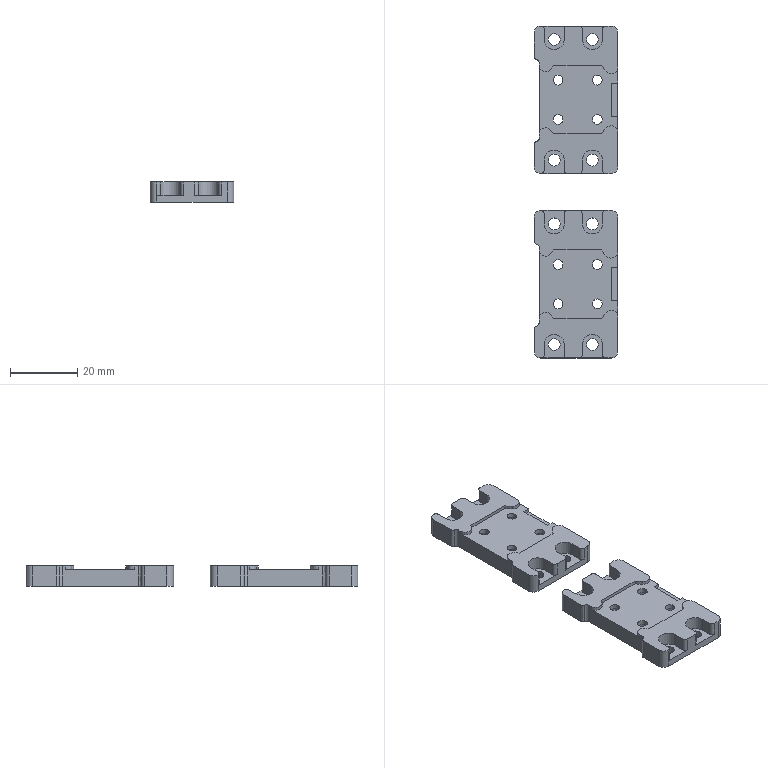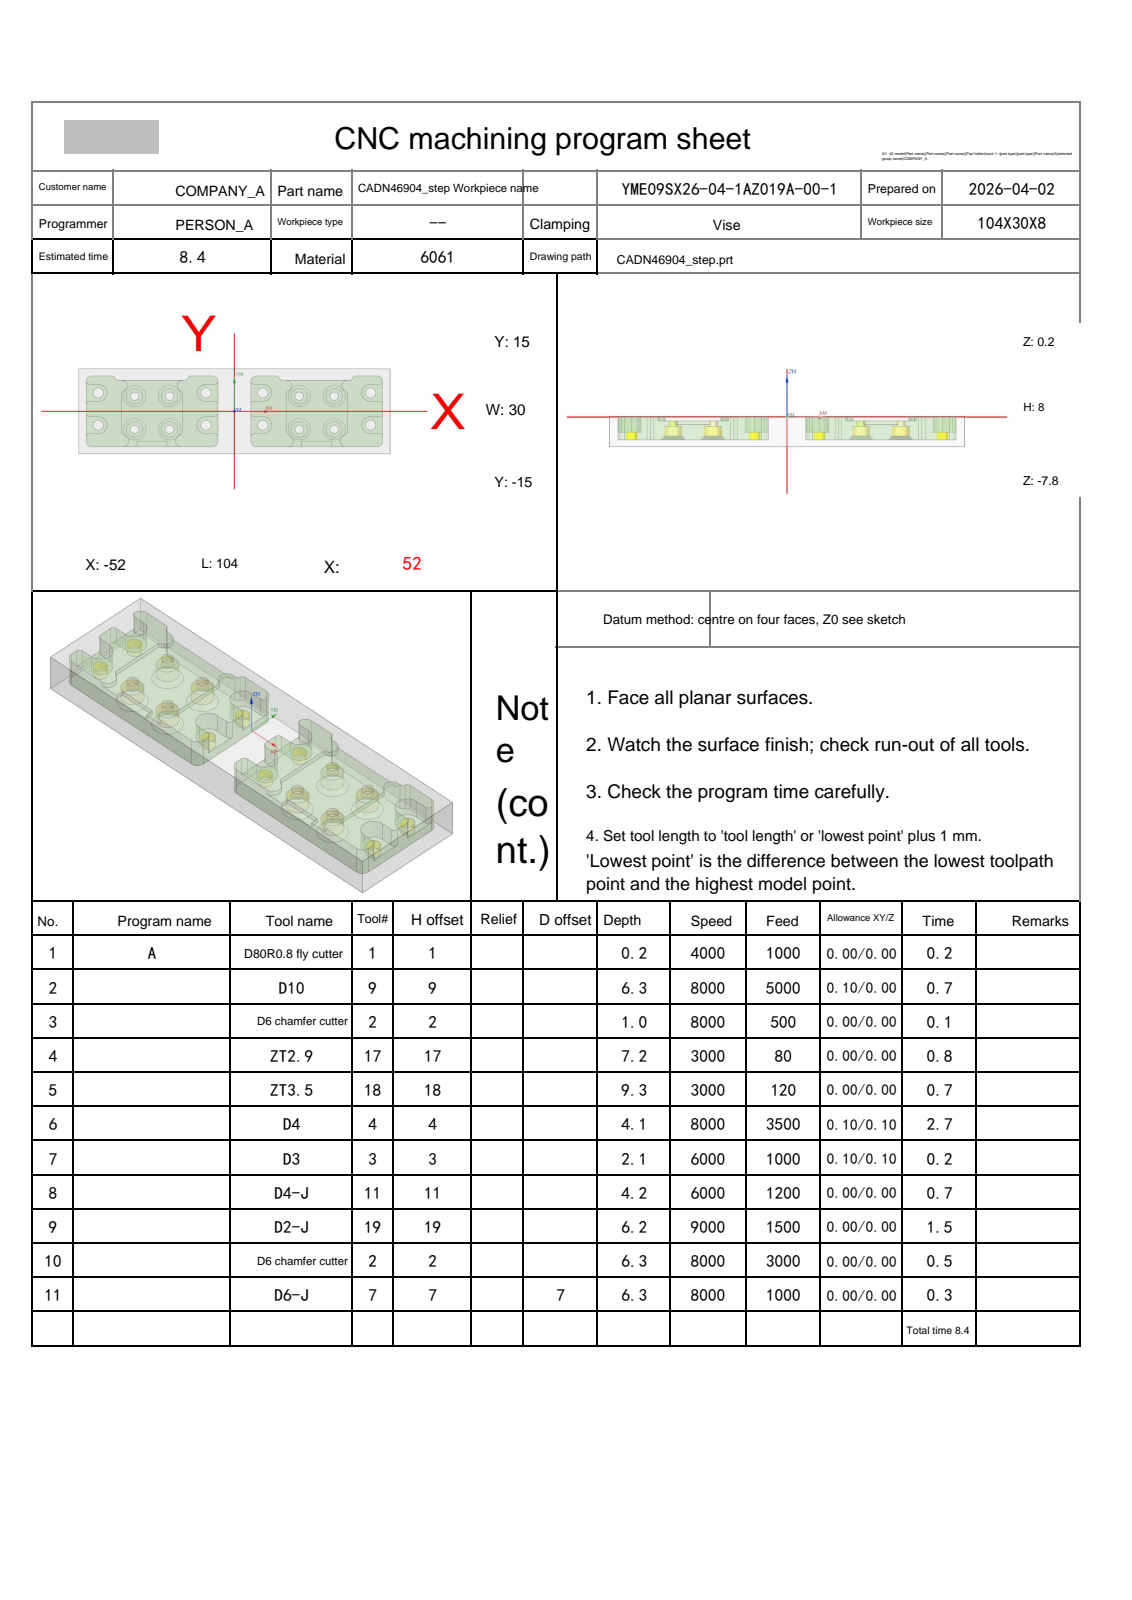NC program | NX | posted by the shop | part box 25 x 99 x 6 mm
Lines 3254 to 4300 of 9316:
N9 T19 M06
(D2-J  D=2. R=0. H=19 ce=0.00 di=0.00)
G00 G90 G54 X31.3 Y-12.7 M03 S8000
G43 H19 Z20.
M08
Z-.9
G01 X31.303 Y-12.699 Z-.93 F800.
X31.31 Y-12.698 Z-.958
X31.321 Y-12.695 Z-.982
X31.335 Y-12.69 Z-1.004
X31.352 Y-12.684 Z-1.023
X31.37 Y-12.676 Z-1.04
X31.39 Y-12.666 Z-1.054
X31.41 Y-12.654 Z-1.066
X31.43 Y-12.64 Z-1.076
X31.448 Y-12.623 Z-1.084
X31.465 Y-12.604 Z-1.09
X31.479 Y-12.582 Z-1.095
X31.49 Y-12.558 Z-1.098
X31.497 Y-12.53 Z-1.099
X31.5 Y-12.5 Z-1.1
Y-11.5
X29.948
X29.921 Y-11.51 Z-1.101
X29.915 Y-11.538 Z-1.102
X29.928 Y-11.582 Z-1.105
X29.957 Y-11.637 Z-1.108
X30. Y-11.702 Z-1.112
X30.056 Y-11.772 Z-1.117
X30.121 Y-11.847 Z-1.122
X30.193 Y-11.921 Z-1.127
X30.412 Y-12.106 Z-1.142
X30.66 Y-12.269 Z-1.158
X30.93 Y-12.404 Z-1.173
X31.033 Y-12.447 Z-1.178
X31.135 Y-12.484 Z-1.183
X31.232 Y-12.514 Z-1.188
X31.318 Y-12.535 Z-1.192
X31.392 Y-12.546 Z-1.195
X31.45 Y-12.544 Z-1.198
X31.487 Y-12.53 Z-1.199
X31.5 Y-12.5 Z-1.2
Y-11.5
X29.947
X29.921 Y-11.51 Z-1.201
X29.915 Y-11.538 Z-1.202
X29.928 Y-11.582 Z-1.205
X29.957 Y-11.637 Z-1.208
X30. Y-11.702 Z-1.212
X30.056 Y-11.772 Z-1.217
X30.12 Y-11.847 Z-1.222
X30.193 Y-11.921 Z-1.227
X30.412 Y-12.106 Z-1.242
X30.66 Y-12.269 Z-1.258
X30.93 Y-12.404 Z-1.273
X31.033 Y-12.447 Z-1.278
X31.135 Y-12.484 Z-1.283
X31.231 Y-12.514 Z-1.288
X31.318 Y-12.535 Z-1.292
X31.392 Y-12.546 Z-1.295
X31.45 Y-12.544 Z-1.298
X31.487 Y-12.53 Z-1.299
X31.5 Y-12.5 Z-1.3
Y-11.5
X29.947
X29.921 Y-11.51 Z-1.301
X29.915 Y-11.538 Z-1.302
X29.928 Y-11.582 Z-1.305
X29.957 Y-11.637 Z-1.308
X30. Y-11.702 Z-1.312
X30.056 Y-11.772 Z-1.317
X30.12 Y-11.847 Z-1.322
X30.193 Y-11.921 Z-1.327
X30.412 Y-12.106 Z-1.342
X30.66 Y-12.269 Z-1.358
X30.93 Y-12.404 Z-1.373
X31.033 Y-12.447 Z-1.378
X31.135 Y-12.484 Z-1.383
X31.231 Y-12.514 Z-1.388
X31.318 Y-12.535 Z-1.392
X31.392 Y-12.546 Z-1.395
X31.45 Y-12.544 Z-1.398
X31.487 Y-12.53 Z-1.399
X31.5 Y-12.5 Z-1.4
Y-11.5
X29.947
X29.921 Y-11.51 Z-1.401
X29.915 Y-11.538 Z-1.402
X29.928 Y-11.582 Z-1.405
X29.957 Y-11.637 Z-1.408
X30. Y-11.702 Z-1.412
X30.055 Y-11.772 Z-1.417
X30.12 Y-11.847 Z-1.422
X30.193 Y-11.921 Z-1.427
X30.412 Y-12.106 Z-1.442
X30.66 Y-12.269 Z-1.458
X30.929 Y-12.404 Z-1.473
X31.033 Y-12.447 Z-1.478
X31.135 Y-12.484 Z-1.483
X31.231 Y-12.514 Z-1.488
X31.318 Y-12.535 Z-1.492
X31.392 Y-12.546 Z-1.495
X31.45 Y-12.544 Z-1.498
X31.487 Y-12.53 Z-1.499
X31.5 Y-12.5 Z-1.5
Y-11.5
X29.947
X29.921 Y-11.51 Z-1.501
X29.915 Y-11.538 Z-1.502
X29.928 Y-11.582 Z-1.505
X29.957 Y-11.637 Z-1.508
X30. Y-11.702 Z-1.512
X30.055 Y-11.772 Z-1.517
X30.12 Y-11.847 Z-1.522
X30.193 Y-11.921 Z-1.527
X30.412 Y-12.106 Z-1.542
X30.66 Y-12.269 Z-1.558
X30.929 Y-12.404 Z-1.573
X31.033 Y-12.447 Z-1.578
X31.135 Y-12.484 Z-1.583
X31.231 Y-12.514 Z-1.588
X31.318 Y-12.535 Z-1.592
X31.392 Y-12.546 Z-1.595
X31.45 Y-12.544 Z-1.598
X31.487 Y-12.53 Z-1.599
X31.5 Y-12.5 Z-1.6
Y-11.5
X29.947
X29.921 Y-11.51 Z-1.601
X29.915 Y-11.538 Z-1.602
X29.928 Y-11.582 Z-1.605
X29.957 Y-11.637 Z-1.608
X30. Y-11.702 Z-1.612
X30.055 Y-11.772 Z-1.617
X30.12 Y-11.847 Z-1.622
X30.193 Y-11.921 Z-1.627
X30.412 Y-12.106 Z-1.642
X30.66 Y-12.269 Z-1.658
X30.929 Y-12.404 Z-1.673
X31.033 Y-12.447 Z-1.678
X31.135 Y-12.484 Z-1.683
X31.231 Y-12.514 Z-1.688
X31.318 Y-12.535 Z-1.692
X31.392 Y-12.546 Z-1.695
X31.45 Y-12.544 Z-1.698
X31.487 Y-12.53 Z-1.699
X31.5 Y-12.5 Z-1.7
Y-11.5
X29.947
X29.921 Y-11.51 Z-1.701
X29.915 Y-11.538 Z-1.702
X29.928 Y-11.582 Z-1.705
X29.957 Y-11.637 Z-1.708
X30. Y-11.702 Z-1.712
X30.055 Y-11.772 Z-1.717
X30.12 Y-11.847 Z-1.722
X30.193 Y-11.921 Z-1.727
X30.412 Y-12.106 Z-1.742
X30.66 Y-12.269 Z-1.758
X30.929 Y-12.404 Z-1.773
X31.033 Y-12.447 Z-1.778
X31.135 Y-12.484 Z-1.783
X31.231 Y-12.514 Z-1.788
X31.318 Y-12.535 Z-1.792
X31.392 Y-12.546 Z-1.795
X31.45 Y-12.544 Z-1.798
X31.487 Y-12.53 Z-1.799
X31.5 Y-12.5 Z-1.8
Y-11.5
X29.947
X29.921 Y-11.51 Z-1.801
X29.915 Y-11.538 Z-1.802
X29.928 Y-11.582 Z-1.805
X29.957 Y-11.637 Z-1.808
X30. Y-11.702 Z-1.812
X30.055 Y-11.772 Z-1.817
X30.12 Y-11.847 Z-1.822
X30.193 Y-11.921 Z-1.827
X30.412 Y-12.106 Z-1.842
X30.66 Y-12.269 Z-1.858
X30.929 Y-12.404 Z-1.873
X31.033 Y-12.447 Z-1.878
X31.135 Y-12.484 Z-1.883
X31.231 Y-12.514 Z-1.888
X31.318 Y-12.535 Z-1.892
X31.392 Y-12.546 Z-1.895
X31.45 Y-12.544 Z-1.898
X31.487 Y-12.53 Z-1.899
X31.5 Y-12.5 Z-1.9
Y-11.5
X29.947
X29.921 Y-11.51 Z-1.901
X29.915 Y-11.538 Z-1.902
X29.928 Y-11.582 Z-1.905
X29.957 Y-11.637 Z-1.908
X30. Y-11.702 Z-1.912
X30.055 Y-11.772 Z-1.917
X30.12 Y-11.847 Z-1.922
X30.193 Y-11.921 Z-1.927
X30.412 Y-12.106 Z-1.942
X30.66 Y-12.269 Z-1.958
X30.929 Y-12.404 Z-1.973
X31.033 Y-12.447 Z-1.978
X31.135 Y-12.484 Z-1.983
X31.231 Y-12.514 Z-1.988
X31.318 Y-12.535 Z-1.992
X31.392 Y-12.546 Z-1.995
X31.45 Y-12.544 Z-1.998
X31.487 Y-12.53 Z-1.999
X31.5 Y-12.5 Z-2.
Y-11.5
X29.946
X29.916 Y-11.503 Z-1.999
X29.888 Y-11.51 Z-1.998
X29.864 Y-11.521 Z-1.995
X29.842 Y-11.535 Z-1.99
X29.823 Y-11.552 Z-1.984
X29.806 Y-11.57 Z-1.976
X29.792 Y-11.59 Z-1.966
X29.78 Y-11.61 Z-1.954
X29.77 Y-11.63 Z-1.94
X29.762 Y-11.648 Z-1.923
X29.756 Y-11.665 Z-1.904
X29.751 Y-11.679 Z-1.882
X29.748 Y-11.69 Z-1.858
X29.747 Y-11.697 Z-1.83
X29.746 Y-11.7 Z-1.8
G00 Z2.
X25.252
Z-.9
G01 Y-11.697 Z-.93
X25.25 Y-11.69 Z-.958
X25.247 Y-11.679 Z-.982
X25.242 Y-11.665 Z-1.004
X25.236 Y-11.648 Z-1.023
X25.228 Y-11.63 Z-1.04
X25.218 Y-11.61 Z-1.054
X25.206 Y-11.59 Z-1.066
X25.192 Y-11.57 Z-1.076
X25.175 Y-11.552 Z-1.084
X25.156 Y-11.535 Z-1.09
X25.135 Y-11.521 Z-1.095
X25.11 Y-11.51 Z-1.098
X25.083 Y-11.503 Z-1.099
X25.052 Y-11.5 Z-1.1
X23.5
Y-12.5
X23.513 Y-12.53 Z-1.101
X23.55 Y-12.544 Z-1.102
X23.608 Y-12.546 Z-1.105
X23.682 Y-12.535 Z-1.108
X23.769 Y-12.514 Z-1.112
X23.865 Y-12.484 Z-1.117
X23.967 Y-12.447 Z-1.122
X24.07 Y-12.404 Z-1.127
X24.34 Y-12.269 Z-1.142
X24.588 Y-12.106 Z-1.158
X24.807 Y-11.921 Z-1.173
X24.88 Y-11.847 Z-1.178
X24.944 Y-11.772 Z-1.183
X25. Y-11.702 Z-1.188
X25.043 Y-11.637 Z-1.192
X25.072 Y-11.582 Z-1.195
X25.085 Y-11.538 Z-1.198
X25.079 Y-11.51 Z-1.199
X25.053 Y-11.5 Z-1.2
X23.5
Y-12.5
X23.513 Y-12.53 Z-1.201
X23.55 Y-12.544 Z-1.202
X23.608 Y-12.546 Z-1.205
X23.682 Y-12.535 Z-1.208
X23.769 Y-12.514 Z-1.212
X23.865 Y-12.484 Z-1.217
X23.967 Y-12.447 Z-1.222
X24.07 Y-12.404 Z-1.227
X24.34 Y-12.269 Z-1.242
X24.588 Y-12.106 Z-1.258
X24.807 Y-11.921 Z-1.273
X24.88 Y-11.847 Z-1.278
X24.944 Y-11.772 Z-1.283
X25. Y-11.702 Z-1.288
X25.043 Y-11.637 Z-1.292
X25.072 Y-11.582 Z-1.295
X25.085 Y-11.538 Z-1.298
X25.079 Y-11.51 Z-1.299
X25.053 Y-11.5 Z-1.3
X23.5
Y-12.5
X23.513 Y-12.53 Z-1.301
X23.55 Y-12.544 Z-1.302
X23.608 Y-12.546 Z-1.305
X23.682 Y-12.535 Z-1.308
X23.769 Y-12.514 Z-1.312
X23.865 Y-12.484 Z-1.317
X23.967 Y-12.447 Z-1.322
X24.071 Y-12.404 Z-1.327
X24.34 Y-12.269 Z-1.342
X24.588 Y-12.106 Z-1.358
X24.807 Y-11.921 Z-1.373
X24.88 Y-11.847 Z-1.378
X24.945 Y-11.772 Z-1.383
X25. Y-11.702 Z-1.388
X25.043 Y-11.637 Z-1.392
X25.072 Y-11.582 Z-1.395
X25.085 Y-11.538 Z-1.398
X25.079 Y-11.51 Z-1.399
X25.053 Y-11.5 Z-1.4
X23.5
Y-12.5
X23.513 Y-12.53 Z-1.401
X23.55 Y-12.544 Z-1.402
X23.608 Y-12.546 Z-1.405
X23.682 Y-12.535 Z-1.408
X23.769 Y-12.514 Z-1.412
X23.865 Y-12.484 Z-1.417
X23.967 Y-12.447 Z-1.422
X24.071 Y-12.404 Z-1.427
X24.34 Y-12.269 Z-1.442
X24.588 Y-12.106 Z-1.458
X24.807 Y-11.921 Z-1.473
X24.88 Y-11.847 Z-1.478
X24.945 Y-11.772 Z-1.483
X25. Y-11.702 Z-1.488
X25.043 Y-11.637 Z-1.492
X25.072 Y-11.582 Z-1.495
X25.085 Y-11.538 Z-1.498
X25.079 Y-11.51 Z-1.499
X25.053 Y-11.5 Z-1.5
X23.5
Y-12.5
X23.513 Y-12.53 Z-1.501
X23.55 Y-12.544 Z-1.502
X23.608 Y-12.546 Z-1.505
X23.682 Y-12.535 Z-1.508
X23.769 Y-12.514 Z-1.512
X23.865 Y-12.484 Z-1.517
X23.967 Y-12.447 Z-1.522
X24.071 Y-12.404 Z-1.527
X24.34 Y-12.269 Z-1.542
X24.588 Y-12.106 Z-1.558
X24.807 Y-11.921 Z-1.573
X24.88 Y-11.847 Z-1.578
X24.945 Y-11.772 Z-1.583
X25. Y-11.702 Z-1.588
X25.043 Y-11.637 Z-1.592
X25.072 Y-11.582 Z-1.595
X25.085 Y-11.538 Z-1.598
X25.079 Y-11.51 Z-1.599
X25.053 Y-11.5 Z-1.6
X23.5
Y-12.5
X23.513 Y-12.53 Z-1.601
X23.55 Y-12.544 Z-1.602
X23.608 Y-12.546 Z-1.605
X23.682 Y-12.535 Z-1.608
X23.769 Y-12.514 Z-1.612
X23.865 Y-12.484 Z-1.617
X23.967 Y-12.447 Z-1.622
X24.071 Y-12.404 Z-1.627
X24.34 Y-12.269 Z-1.642
X24.588 Y-12.106 Z-1.658
X24.807 Y-11.921 Z-1.673
X24.88 Y-11.847 Z-1.678
X24.945 Y-11.772 Z-1.683
X25. Y-11.702 Z-1.688
X25.043 Y-11.637 Z-1.692
X25.072 Y-11.582 Z-1.695
X25.085 Y-11.538 Z-1.698
X25.079 Y-11.51 Z-1.699
X25.053 Y-11.5 Z-1.7
X23.5
Y-12.5
X23.513 Y-12.53 Z-1.701
X23.55 Y-12.544 Z-1.702
X23.608 Y-12.546 Z-1.705
X23.682 Y-12.535 Z-1.708
X23.769 Y-12.514 Z-1.712
X23.865 Y-12.484 Z-1.717
X23.967 Y-12.447 Z-1.722
X24.071 Y-12.404 Z-1.727
X24.34 Y-12.269 Z-1.742
X24.588 Y-12.106 Z-1.758
X24.807 Y-11.921 Z-1.773
X24.88 Y-11.847 Z-1.778
X24.945 Y-11.772 Z-1.783
X25. Y-11.702 Z-1.788
X25.043 Y-11.637 Z-1.792
X25.072 Y-11.582 Z-1.795
X25.085 Y-11.538 Z-1.798
X25.079 Y-11.51 Z-1.799
X25.053 Y-11.5 Z-1.8
X23.5
Y-12.5
X23.513 Y-12.53 Z-1.801
X23.55 Y-12.544 Z-1.802
X23.608 Y-12.546 Z-1.805
X23.682 Y-12.535 Z-1.808
X23.769 Y-12.514 Z-1.812
X23.865 Y-12.484 Z-1.817
X23.967 Y-12.447 Z-1.822
X24.071 Y-12.404 Z-1.827
X24.34 Y-12.269 Z-1.842
X24.588 Y-12.106 Z-1.858
X24.807 Y-11.921 Z-1.873
X24.88 Y-11.847 Z-1.878
X24.945 Y-11.772 Z-1.883
X25. Y-11.702 Z-1.888
X25.043 Y-11.637 Z-1.892
X25.072 Y-11.582 Z-1.895
X25.085 Y-11.538 Z-1.898
X25.079 Y-11.51 Z-1.899
X25.053 Y-11.5 Z-1.9
X23.5
Y-12.357
X23.513 Y-12.387 Z-1.901
X23.55 Y-12.404 Z-1.902
X23.608 Y-12.409 Z-1.905
X23.682 Y-12.403 Z-1.908
X23.769 Y-12.388 Z-1.912
X23.865 Y-12.365 Z-1.917
X23.967 Y-12.335 Z-1.922
X24.071 Y-12.3 Z-1.927
X24.274 Y-12.217 Z-1.938
X24.468 Y-12.119 Z-1.95
X24.647 Y-12.007 Z-1.962
X24.808 Y-11.882 Z-1.973
X24.881 Y-11.815 Z-1.978
X24.946 Y-11.749 Z-1.983
X25.001 Y-11.684 Z-1.988
X25.044 Y-11.625 Z-1.992
X25.073 Y-11.575 Z-1.995
X25.086 Y-11.535 Z-1.998
X25.08 Y-11.509 Z-1.999
X25.054 Y-11.5 Z-2.
X23.5
Y-12.357
X23.503 Y-12.387 Z-1.999
X23.51 Y-12.415 Z-1.998
X23.521 Y-12.439 Z-1.995
X23.535 Y-12.461 Z-1.99
X23.552 Y-12.48 Z-1.984
X23.57 Y-12.496 Z-1.976
X23.59 Y-12.511 Z-1.966
X23.61 Y-12.523 Z-1.954
X23.63 Y-12.533 Z-1.94
X23.648 Y-12.541 Z-1.923
X23.665 Y-12.547 Z-1.904
X23.679 Y-12.552 Z-1.882
X23.69 Y-12.555 Z-1.858
X23.697 Y-12.556 Z-1.83
X23.7 Y-12.557 Z-1.8
G00 Z20.
X-23.7 Y-12.7
Z-.9
G01 X-23.697 Y-12.699 Z-.93
X-23.69 Y-12.698 Z-.958
X-23.679 Y-12.695 Z-.982
X-23.665 Y-12.69 Z-1.004
X-23.648 Y-12.684 Z-1.023
X-23.63 Y-12.676 Z-1.04
X-23.61 Y-12.666 Z-1.054
X-23.59 Y-12.654 Z-1.066
X-23.57 Y-12.64 Z-1.076
X-23.552 Y-12.623 Z-1.084
X-23.535 Y-12.604 Z-1.09
X-23.521 Y-12.582 Z-1.095
X-23.51 Y-12.558 Z-1.098
X-23.503 Y-12.53 Z-1.099
X-23.5 Y-12.5 Z-1.1
Y-11.5
X-25.052
X-25.079 Y-11.51 Z-1.101
X-25.085 Y-11.538 Z-1.102
X-25.072 Y-11.582 Z-1.105
X-25.043 Y-11.637 Z-1.108
X-25. Y-11.702 Z-1.112
X-24.944 Y-11.772 Z-1.117
X-24.879 Y-11.847 Z-1.122
X-24.807 Y-11.921 Z-1.127
X-24.588 Y-12.106 Z-1.142
X-24.34 Y-12.269 Z-1.158
X-24.07 Y-12.404 Z-1.173
X-23.967 Y-12.447 Z-1.178
X-23.865 Y-12.484 Z-1.183
X-23.768 Y-12.514 Z-1.188
X-23.682 Y-12.535 Z-1.192
X-23.608 Y-12.546 Z-1.195
X-23.55 Y-12.544 Z-1.198
X-23.513 Y-12.53 Z-1.199
X-23.5 Y-12.5 Z-1.2
Y-11.5
X-25.053
X-25.079 Y-11.51 Z-1.201
X-25.085 Y-11.538 Z-1.202
X-25.072 Y-11.582 Z-1.205
X-25.043 Y-11.637 Z-1.208
X-25. Y-11.702 Z-1.212
X-24.944 Y-11.772 Z-1.217
X-24.88 Y-11.847 Z-1.222
X-24.807 Y-11.921 Z-1.227
X-24.588 Y-12.106 Z-1.242
X-24.34 Y-12.269 Z-1.258
X-24.07 Y-12.404 Z-1.273
X-23.967 Y-12.447 Z-1.278
X-23.865 Y-12.484 Z-1.283
X-23.769 Y-12.514 Z-1.288
X-23.682 Y-12.535 Z-1.292
X-23.608 Y-12.546 Z-1.295
X-23.55 Y-12.544 Z-1.298
X-23.513 Y-12.53 Z-1.299
X-23.5 Y-12.5 Z-1.3
Y-11.5
X-25.053
X-25.079 Y-11.51 Z-1.301
X-25.085 Y-11.538 Z-1.302
X-25.072 Y-11.582 Z-1.305
X-25.043 Y-11.637 Z-1.308
X-25. Y-11.702 Z-1.312
X-24.944 Y-11.772 Z-1.317
X-24.88 Y-11.847 Z-1.322
X-24.807 Y-11.921 Z-1.327
X-24.588 Y-12.106 Z-1.342
X-24.34 Y-12.269 Z-1.358
X-24.07 Y-12.404 Z-1.373
X-23.967 Y-12.447 Z-1.378
X-23.865 Y-12.484 Z-1.383
X-23.769 Y-12.514 Z-1.388
X-23.682 Y-12.535 Z-1.392
X-23.608 Y-12.546 Z-1.395
X-23.55 Y-12.544 Z-1.398
X-23.513 Y-12.53 Z-1.399
X-23.5 Y-12.5 Z-1.4
Y-11.5
X-25.053
X-25.079 Y-11.51 Z-1.401
X-25.085 Y-11.538 Z-1.402
X-25.072 Y-11.582 Z-1.405
X-25.043 Y-11.637 Z-1.408
X-25. Y-11.702 Z-1.412
X-24.945 Y-11.772 Z-1.417
X-24.88 Y-11.847 Z-1.422
X-24.807 Y-11.921 Z-1.427
X-24.588 Y-12.106 Z-1.442
X-24.34 Y-12.269 Z-1.458
X-24.071 Y-12.404 Z-1.473
X-23.967 Y-12.447 Z-1.478
X-23.865 Y-12.484 Z-1.483
X-23.769 Y-12.514 Z-1.488
X-23.682 Y-12.535 Z-1.492
X-23.608 Y-12.546 Z-1.495
X-23.55 Y-12.544 Z-1.498
X-23.513 Y-12.53 Z-1.499
X-23.5 Y-12.5 Z-1.5
Y-11.5
X-25.053
X-25.079 Y-11.51 Z-1.501
X-25.085 Y-11.538 Z-1.502
X-25.072 Y-11.582 Z-1.505
X-25.043 Y-11.637 Z-1.508
X-25. Y-11.702 Z-1.512
X-24.945 Y-11.772 Z-1.517
X-24.88 Y-11.847 Z-1.522
X-24.807 Y-11.921 Z-1.527
X-24.588 Y-12.106 Z-1.542
X-24.34 Y-12.269 Z-1.558
X-24.071 Y-12.404 Z-1.573
X-23.967 Y-12.447 Z-1.578
X-23.865 Y-12.484 Z-1.583
X-23.769 Y-12.514 Z-1.588
X-23.682 Y-12.535 Z-1.592
X-23.608 Y-12.546 Z-1.595
X-23.55 Y-12.544 Z-1.598
X-23.513 Y-12.53 Z-1.599
X-23.5 Y-12.5 Z-1.6
Y-11.5
X-25.053
X-25.079 Y-11.51 Z-1.601
X-25.085 Y-11.538 Z-1.602
X-25.072 Y-11.582 Z-1.605
X-25.043 Y-11.637 Z-1.608
X-25. Y-11.702 Z-1.612
X-24.945 Y-11.772 Z-1.617
X-24.88 Y-11.847 Z-1.622
X-24.807 Y-11.921 Z-1.627
X-24.588 Y-12.106 Z-1.642
X-24.34 Y-12.269 Z-1.658
X-24.071 Y-12.404 Z-1.673
X-23.967 Y-12.447 Z-1.678
X-23.865 Y-12.484 Z-1.683
X-23.769 Y-12.514 Z-1.688
X-23.682 Y-12.535 Z-1.692
X-23.608 Y-12.546 Z-1.695
X-23.55 Y-12.544 Z-1.698
X-23.513 Y-12.53 Z-1.699
X-23.5 Y-12.5 Z-1.7
Y-11.5
X-25.053
X-25.079 Y-11.51 Z-1.701
X-25.085 Y-11.538 Z-1.702
X-25.072 Y-11.582 Z-1.705
X-25.043 Y-11.637 Z-1.708
X-25. Y-11.702 Z-1.712
X-24.945 Y-11.772 Z-1.717
X-24.88 Y-11.847 Z-1.722
X-24.807 Y-11.921 Z-1.727
X-24.588 Y-12.106 Z-1.742
X-24.34 Y-12.269 Z-1.758
X-24.071 Y-12.404 Z-1.773
X-23.967 Y-12.447 Z-1.778
X-23.865 Y-12.484 Z-1.783
X-23.769 Y-12.514 Z-1.788
X-23.682 Y-12.535 Z-1.792
X-23.608 Y-12.546 Z-1.795
X-23.55 Y-12.544 Z-1.798
X-23.513 Y-12.53 Z-1.799
X-23.5 Y-12.5 Z-1.8
Y-11.5
X-25.053
X-25.079 Y-11.51 Z-1.801
X-25.085 Y-11.538 Z-1.802
X-25.072 Y-11.582 Z-1.805
X-25.043 Y-11.637 Z-1.808
X-25. Y-11.702 Z-1.812
X-24.945 Y-11.772 Z-1.817
X-24.88 Y-11.847 Z-1.822
X-24.807 Y-11.921 Z-1.827
X-24.588 Y-12.106 Z-1.842
X-24.34 Y-12.269 Z-1.858
X-24.071 Y-12.404 Z-1.873
X-23.967 Y-12.447 Z-1.878
X-23.865 Y-12.484 Z-1.883
X-23.769 Y-12.514 Z-1.888
X-23.682 Y-12.535 Z-1.892
X-23.608 Y-12.546 Z-1.895
X-23.55 Y-12.544 Z-1.898
X-23.513 Y-12.53 Z-1.899
X-23.5 Y-12.5 Z-1.9
Y-11.5
X-25.053
X-25.079 Y-11.51 Z-1.901
X-25.085 Y-11.538 Z-1.902
X-25.072 Y-11.582 Z-1.905
X-25.043 Y-11.637 Z-1.908
X-25. Y-11.702 Z-1.912
X-24.945 Y-11.772 Z-1.917
X-24.88 Y-11.847 Z-1.922
X-24.807 Y-11.921 Z-1.927
X-24.588 Y-12.106 Z-1.942
X-24.34 Y-12.269 Z-1.958
X-24.071 Y-12.404 Z-1.973
X-23.967 Y-12.447 Z-1.978
X-23.865 Y-12.484 Z-1.983
X-23.769 Y-12.514 Z-1.988
X-23.682 Y-12.535 Z-1.992
X-23.608 Y-12.546 Z-1.995
X-23.55 Y-12.544 Z-1.998
X-23.513 Y-12.53 Z-1.999
X-23.5 Y-12.5 Z-2.
Y-11.5
X-25.054
X-25.084 Y-11.503 Z-1.999
X-25.112 Y-11.51 Z-1.998
X-25.136 Y-11.521 Z-1.995
X-25.158 Y-11.535 Z-1.99
X-25.177 Y-11.552 Z-1.984
X-25.194 Y-11.57 Z-1.976
X-25.208 Y-11.59 Z-1.966
X-25.22 Y-11.61 Z-1.954
X-25.23 Y-11.63 Z-1.94
X-25.238 Y-11.648 Z-1.923
X-25.244 Y-11.665 Z-1.904
X-25.249 Y-11.679 Z-1.882
X-25.252 Y-11.69 Z-1.858
X-25.253 Y-11.697 Z-1.83
X-25.254 Y-11.7 Z-1.8
G00 Z2.
X-29.748
Z-.9
G01 Y-11.697 Z-.93
X-29.75 Y-11.69 Z-.958
X-29.753 Y-11.679 Z-.982
X-29.758 Y-11.665 Z-1.004
X-29.764 Y-11.648 Z-1.023
X-29.772 Y-11.63 Z-1.04
X-29.782 Y-11.61 Z-1.054
X-29.794 Y-11.59 Z-1.066
X-29.808 Y-11.57 Z-1.076
X-29.825 Y-11.552 Z-1.084
X-29.844 Y-11.535 Z-1.09
X-29.865 Y-11.521 Z-1.095
X-29.89 Y-11.51 Z-1.098
X-29.917 Y-11.503 Z-1.099
X-29.948 Y-11.5 Z-1.1
X-31.5
Y-12.5
X-31.487 Y-12.53 Z-1.101
X-31.45 Y-12.544 Z-1.102
X-31.392 Y-12.546 Z-1.105
X-31.318 Y-12.535 Z-1.108
X-31.231 Y-12.514 Z-1.112
X-31.135 Y-12.484 Z-1.117
X-31.033 Y-12.447 Z-1.122
X-30.93 Y-12.404 Z-1.127
X-30.66 Y-12.269 Z-1.142
X-30.412 Y-12.106 Z-1.158
X-30.193 Y-11.921 Z-1.173
X-30.12 Y-11.847 Z-1.178
X-30.056 Y-11.772 Z-1.183
X-30. Y-11.702 Z-1.188
X-29.957 Y-11.637 Z-1.192
X-29.928 Y-11.582 Z-1.195
X-29.915 Y-11.538 Z-1.198
X-29.921 Y-11.51 Z-1.199
X-29.947 Y-11.5 Z-1.2
X-31.5
Y-12.5
X-31.487 Y-12.53 Z-1.201
X-31.45 Y-12.544 Z-1.202
X-31.392 Y-12.546 Z-1.205
X-31.318 Y-12.535 Z-1.208
X-31.231 Y-12.514 Z-1.212
X-31.135 Y-12.484 Z-1.217
X-31.033 Y-12.447 Z-1.222
X-30.93 Y-12.404 Z-1.227
X-30.66 Y-12.269 Z-1.242
X-30.412 Y-12.106 Z-1.258
X-30.193 Y-11.921 Z-1.273
X-30.12 Y-11.847 Z-1.278
X-30.056 Y-11.772 Z-1.283
X-30. Y-11.702 Z-1.288
X-29.957 Y-11.637 Z-1.292
X-29.928 Y-11.582 Z-1.295
X-29.915 Y-11.538 Z-1.298
X-29.921 Y-11.51 Z-1.299
X-29.947 Y-11.5 Z-1.3
X-31.5
Y-12.5
X-31.487 Y-12.53 Z-1.301
X-31.45 Y-12.544 Z-1.302
X-31.392 Y-12.546 Z-1.305
X-31.318 Y-12.535 Z-1.308
X-31.231 Y-12.514 Z-1.312
X-31.135 Y-12.484 Z-1.317
X-31.033 Y-12.447 Z-1.322
X-30.929 Y-12.404 Z-1.327
X-30.66 Y-12.269 Z-1.342
X-30.412 Y-12.106 Z-1.358
X-30.193 Y-11.921 Z-1.373
X-30.12 Y-11.847 Z-1.378
X-30.055 Y-11.772 Z-1.383
X-30. Y-11.702 Z-1.388
X-29.957 Y-11.637 Z-1.392
X-29.928 Y-11.582 Z-1.395
X-29.915 Y-11.538 Z-1.398
X-29.921 Y-11.51 Z-1.399
X-29.947 Y-11.5 Z-1.4
X-31.5
Y-12.5
X-31.487 Y-12.53 Z-1.401
X-31.45 Y-12.544 Z-1.402
X-31.392 Y-12.546 Z-1.405
X-31.318 Y-12.535 Z-1.408
X-31.231 Y-12.514 Z-1.412
X-31.135 Y-12.484 Z-1.417
X-31.033 Y-12.447 Z-1.422
X-30.929 Y-12.404 Z-1.427
X-30.66 Y-12.269 Z-1.442
X-30.412 Y-12.106 Z-1.458
X-30.193 Y-11.921 Z-1.473
X-30.12 Y-11.847 Z-1.478
X-30.055 Y-11.772 Z-1.483
X-30. Y-11.702 Z-1.488
X-29.957 Y-11.637 Z-1.492
X-29.928 Y-11.582 Z-1.495
X-29.915 Y-11.538 Z-1.498
X-29.921 Y-11.51 Z-1.499
X-29.947 Y-11.5 Z-1.5
X-31.5
Y-12.5
X-31.487 Y-12.53 Z-1.501
X-31.45 Y-12.544 Z-1.502
X-31.392 Y-12.546 Z-1.505
X-31.318 Y-12.535 Z-1.508
X-31.231 Y-12.514 Z-1.512
X-31.135 Y-12.484 Z-1.517
X-31.033 Y-12.447 Z-1.522
X-30.929 Y-12.404 Z-1.527
X-30.66 Y-12.269 Z-1.542
X-30.412 Y-12.106 Z-1.558
X-30.193 Y-11.921 Z-1.573
X-30.12 Y-11.847 Z-1.578
X-30.055 Y-11.772 Z-1.583
X-30. Y-11.702 Z-1.588
X-29.957 Y-11.637 Z-1.592
X-29.928 Y-11.582 Z-1.595
X-29.915 Y-11.538 Z-1.598
X-29.921 Y-11.51 Z-1.599
X-29.947 Y-11.5 Z-1.6
X-31.5
Y-12.5
X-31.487 Y-12.53 Z-1.601
X-31.45 Y-12.544 Z-1.602
X-31.392 Y-12.546 Z-1.605
X-31.318 Y-12.535 Z-1.608
X-31.231 Y-12.514 Z-1.612
X-31.135 Y-12.484 Z-1.617
X-31.033 Y-12.447 Z-1.622
X-30.929 Y-12.404 Z-1.627
X-30.66 Y-12.269 Z-1.642
X-30.412 Y-12.106 Z-1.658
X-30.193 Y-11.921 Z-1.673
X-30.12 Y-11.847 Z-1.678
X-30.055 Y-11.772 Z-1.683
X-30. Y-11.702 Z-1.688
X-29.957 Y-11.637 Z-1.692
X-29.928 Y-11.582 Z-1.695
X-29.915 Y-11.538 Z-1.698
X-29.921 Y-11.51 Z-1.699
X-29.947 Y-11.5 Z-1.7
X-31.5
Y-12.5
X-31.487 Y-12.53 Z-1.701
X-31.45 Y-12.544 Z-1.702
X-31.392 Y-12.546 Z-1.705
X-31.318 Y-12.535 Z-1.708
X-31.231 Y-12.514 Z-1.712
X-31.135 Y-12.484 Z-1.717
X-31.033 Y-12.447 Z-1.722
X-30.929 Y-12.404 Z-1.727
X-30.66 Y-12.269 Z-1.742
X-30.412 Y-12.106 Z-1.758
X-30.193 Y-11.921 Z-1.773
X-30.12 Y-11.847 Z-1.778
X-30.055 Y-11.772 Z-1.783
X-30. Y-11.702 Z-1.788
X-29.957 Y-11.637 Z-1.792
X-29.928 Y-11.582 Z-1.795
X-29.915 Y-11.538 Z-1.798
X-29.921 Y-11.51 Z-1.799
X-29.947 Y-11.5 Z-1.8
X-31.5
Y-12.5
X-31.487 Y-12.53 Z-1.801
X-31.45 Y-12.544 Z-1.802
X-31.392 Y-12.546 Z-1.805
X-31.318 Y-12.535 Z-1.808
X-31.231 Y-12.514 Z-1.812
X-31.135 Y-12.484 Z-1.817
X-31.033 Y-12.447 Z-1.822
X-30.929 Y-12.404 Z-1.827
X-30.66 Y-12.269 Z-1.842
X-30.412 Y-12.106 Z-1.858
X-30.193 Y-11.921 Z-1.873
X-30.12 Y-11.847 Z-1.878
X-30.055 Y-11.772 Z-1.883
X-30. Y-11.702 Z-1.888
X-29.957 Y-11.637 Z-1.892
X-29.928 Y-11.582 Z-1.895
X-29.915 Y-11.538 Z-1.898
X-29.921 Y-11.51 Z-1.899
X-29.947 Y-11.5 Z-1.9
X-31.5
Y-12.5
X-31.487 Y-12.53 Z-1.901
X-31.45 Y-12.544 Z-1.902
X-31.392 Y-12.546 Z-1.905
X-31.318 Y-12.535 Z-1.908
X-31.231 Y-12.514 Z-1.912
X-31.135 Y-12.484 Z-1.917
X-31.033 Y-12.447 Z-1.922
X-30.929 Y-12.404 Z-1.927
X-30.66 Y-12.269 Z-1.942
X-30.411 Y-12.106 Z-1.958
X-30.192 Y-11.921 Z-1.973
X-30.119 Y-11.847 Z-1.978
X-30.054 Y-11.772 Z-1.983
X-29.999 Y-11.702 Z-1.988
X-29.956 Y-11.637 Z-1.992
X-29.927 Y-11.582 Z-1.995
X-29.914 Y-11.538 Z-1.998
X-29.92 Y-11.51 Z-1.999
X-29.946 Y-11.5 Z-2.
X-31.5
Y-12.5
X-31.497 Y-12.53 Z-1.999
X-31.49 Y-12.558 Z-1.998
X-31.479 Y-12.582 Z-1.995
X-31.465 Y-12.604 Z-1.99
X-31.448 Y-12.623 Z-1.984
X-31.43 Y-12.64 Z-1.976
X-31.41 Y-12.654 Z-1.966
X-31.39 Y-12.666 Z-1.954
X-31.37 Y-12.676 Z-1.94
X-31.352 Y-12.684 Z-1.923
X-31.335 Y-12.69 Z-1.904
X-31.321 Y-12.695 Z-1.882
X-31.31 Y-12.698 Z-1.858
X-31.303 Y-12.699 Z-1.83
X-31.3 Y-12.7 Z-1.8
G00 Z20.
G00 G90 X15.028 Y14.182 M03 S9000
Z20.
Z.552
G01 X15.025 Y14.173 Z.438 F1200.
X15.015 Y14.147 Z.335
X15. Y14.106 Z.243
X14.984 Y14.052 Z.162
X14.967 Y13.987 Z.091
X14.952 Y13.913 Z.028
X14.94 Y13.831 Z-.025
X14.934 Y13.744 Z-.07
X14.935 Y13.653 Z-.107
X14.946 Y13.56 Z-.137
X14.968 Y13.468 Z-.161
X15.004 Y13.377 Z-.178
X15.055 Y13.29 Z-.19
X15.124 Y13.209 Z-.196
X15.212 Y13.136 Z-.198
G02 X16. Y12. I-1.152 J-1.64 F1500.
G01 X17.153
X17.176 Y12.013 Z-.199
X17.173 Y12.051 Z-.203
X17.145 Y12.108 Z-.208
X17.097 Y12.181 Z-.214
X17.03 Y12.266 Z-.222
X16.948 Y12.358 Z-.231
X16.854 Y12.454 Z-.241
X16.751 Y12.549 Z-.252
X16.524 Y12.726 Z-.274
X16.281 Y12.88 Z-.297
X16.028 Y13.005 Z-.321
X15.775 Y13.097 Z-.343
X15.652 Y13.129 Z-.354
X15.535 Y13.153 Z-.364
X15.429 Y13.168 Z-.373
X15.338 Y13.175 Z-.381
X15.266 Z-.387
X15.219 Y13.168 Z-.392
X15.199 Y13.155 Z-.396
X15.212 Y13.136 Z-.397
G02 X16. Y12. I-1.152 J-1.64
G01 X17.153
X17.176 Y12.013 Z-.398
X17.172 Y12.051 Z-.401
X17.144 Y12.109 Z-.406
X17.095 Y12.182 Z-.413
X17.027 Y12.267 Z-.421
X16.944 Y12.36 Z-.43
X16.849 Y12.457 Z-.44
X16.744 Y12.553 Z-.45
X16.515 Y12.732 Z-.473
X16.268 Y12.887 Z-.496
X16.013 Y13.014 Z-.519
X15.758 Y13.107 Z-.541
X15.634 Y13.14 Z-.552
X15.516 Y13.164 Z-.562
X15.409 Y13.18 Z-.571
X15.318 Y13.188 Z-.579
X15.246 Z-.586
X15.198 Y13.182 Z-.591
X15.178 Y13.169 Z-.594
X15.191 Y13.15 Z-.595
G02 X16. Y12. I-1.131 J-1.654
G01 X17.153
X17.176 Y12.013 Z-.596
X17.172 Y12.051 Z-.599
X17.144 Y12.109 Z-.604
X17.095 Y12.182 Z-.611
X17.027 Y12.268 Z-.619
X16.944 Y12.361 Z-.628
X16.848 Y12.457 Z-.638
X16.743 Y12.553 Z-.649
X16.514 Y12.732 Z-.671
X16.268 Y12.887 Z-.694
X16.013 Y13.014 Z-.717
X15.757 Y13.108 Z-.74
X15.633 Y13.141 Z-.75
X15.515 Y13.165 Z-.76
X15.408 Y13.18 Z-.769
X15.317 Y13.188 Z-.777
X15.245 Y13.189 Z-.784
X15.197 Y13.182 Z-.789
X15.177 Y13.169 Z-.792
X15.19 Y13.151 Z-.793
G02 X16. Y12. I-1.13 J-1.655
G01 X17.153
X17.176 Y12.013 Z-.794
X17.172 Y12.051 Z-.798
X17.144 Y12.109 Z-.803
X17.095 Y12.182 Z-.809
X17.027 Y12.267 Z-.817
X16.944 Y12.36 Z-.826
X16.849 Y12.457 Z-.836
X16.744 Y12.553 Z-.847
X16.515 Y12.731 Z-.869
X16.269 Y12.887 Z-.892
X16.014 Y13.013 Z-.916
X15.759 Y13.107 Z-.938
X15.635 Y13.14 Z-.949
X15.517 Y13.164 Z-.959
X15.41 Y13.179 Z-.968
X15.318 Y13.187 Z-.976
X15.247 Z-.982
X15.199 Y13.181 Z-.987
X15.179 Y13.168 Z-.991
X15.192 Y13.15 Z-.992
G02 X16. Y12. I-1.132 J-1.654
G01 X17.153
X17.176 Y12.014 Z-.993
X17.171 Y12.052 Z-.996
X17.142 Y12.11 Z-1.001
X17.091 Y12.184 Z-1.008
X17.022 Y12.27 Z-1.016
X16.937 Y12.364 Z-1.025
X16.84 Y12.462 Z-1.035
X16.733 Y12.559 Z-1.045
X16.499 Y12.74 Z-1.068
X16.248 Y12.898 Z-1.091
X15.988 Y13.027 Z-1.114
X15.729 Y13.123 Z-1.136
X15.604 Y13.157 Z-1.147
X15.484 Y13.182 Z-1.157
X15.377 Y13.199 Z-1.166
X15.284 Y13.208 Z-1.174
X15.212 Y13.209 Z-1.181
X15.163 Y13.203 Z-1.186
X15.144 Y13.191 Z-1.189
X15.157 Y13.173 Z-1.19
G02 X16. Y12. I-1.097 J-1.677
G01 X18.135
X18.152 Y12.011 Z-1.191
X18.139 Y12.041 Z-1.193
X18.099 Y12.088 Z-1.197
X18.034 Y12.149 Z-1.203
X17.948 Y12.221 Z-1.209
X17.843 Y12.301 Z-1.217
X17.723 Y12.386 Z-1.225
X17.591 Y12.473 Z-1.234
X17.448 Y12.559 Z-1.244
X17.104 Y12.74 Z-1.266
X16.739 Y12.898 Z-1.289
X16.365 Y13.027 Z-1.312
X15.995 Y13.123 Z-1.335
X15.836 Y13.154 Z-1.344
X15.685 Y13.178 Z-1.353
X15.544 Y13.194 Z-1.361